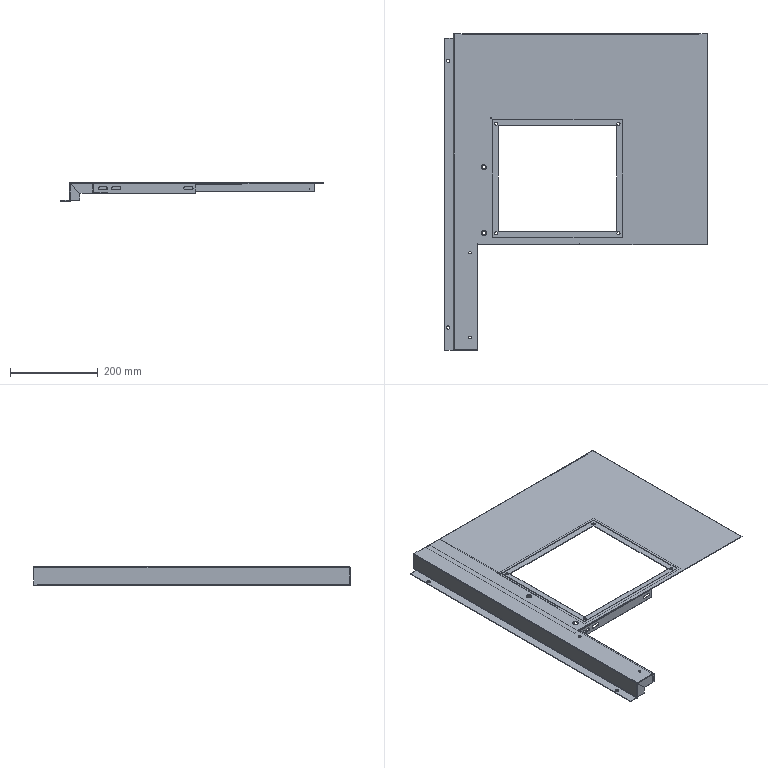Part | SolidWorks | 3 solids | 181 faces | box 600 x 723 x 41.7 mm | volume 569588 mm3 | plane 119 | cylinder 60 | spline 2 | commonest cylinder face diameters 0.4 x9 2 x8 6 x8 7.1 x8 3.4 x6 7 x6